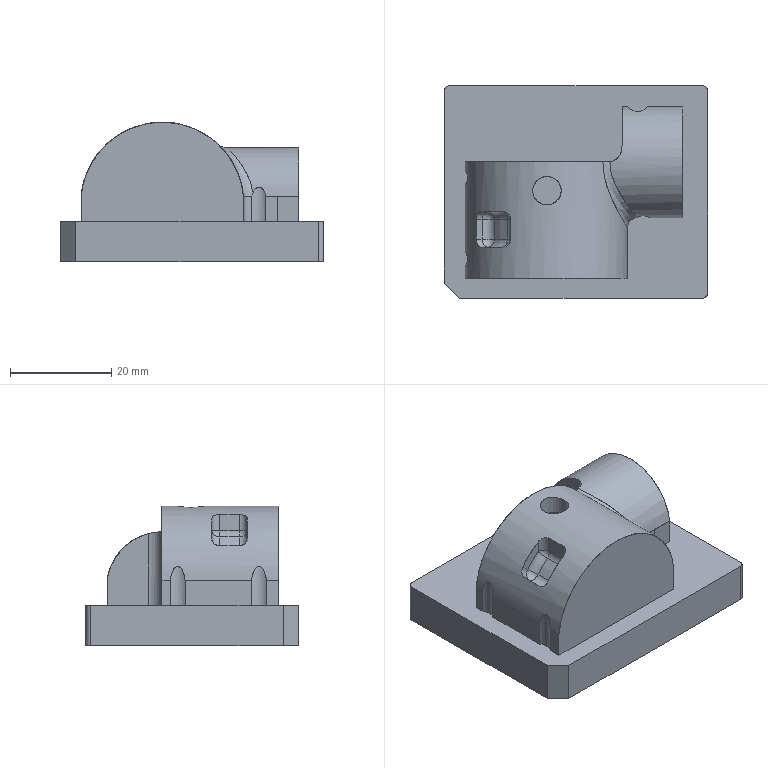CAM job | PowerMill | 3-axis milling, other | part box 52 x 42 x 27.622 mm
Tools:
number,name,type,diameter,tip_radius,length,cutting_length,overhang,flutes,holder,toolpaths_using
1,D10C,end_mill,10.0,0.0,60.0,,30.0,1,D42L35,2
2,D4C,end_mill,4.0,0.0,30.0,,15.0,1,D42L35,2
1,D10C_1_1_1,end_mill,10.0,0.0,60.0,,28.08,1,D42L35,3
2,D4C_1_1,end_mill,4.0,0.0,30.0,,19.8,1,D42L35,2
28,D2C_1_1,end_mill,2.0,0.0,4.16,,12.72,1,D42L35,1
3,D10_1_1_1,end_mill,10.0,0.0,60.0,,27.8,1,D42L35,6
7,R2_1_1,ball_nosed,4.0,2.0,30.0,,16.76,1,D42L35,1
10,D3_1_1,end_mill,3.0,0.0,30.0,,19.88,1,D42L35,1
4,R1_1_1,ball_nosed,2.0,1.0,5.0,,9.72,1,D42L35,2
13,Text_D4_1_1,taper_spherical,4.0,0.3,60.0,,19.88,1,D42L35,2
1,D10C_2_1_1,end_mill,10.0,0.0,60.0,,28.08,1,D42L35,3
2,D4C_2_1,end_mill,4.0,0.0,30.0,,19.68,1,D42L35,2
28,D2C_2_1,end_mill,2.0,0.0,4.24,,9.8,1,D42L35,1
7,R2_2_1,ball_nosed,4.0,2.0,30.0,,16.6,1,D42L35,1
10,D3_2_1,end_mill,3.0,0.0,30.0,,19.76,1,D42L35,1
Operations:
program,toolpath,strategy,tool,tool_number,tool_diameter,tip_radius,flutes,spindle_rpm,feed_cut,surface_speed_m_min_computed,feed_per_tooth_computed,tolerance,thickness,stepover,stepdown,cut_length,cut_time_min,total_time_min,workplane
04-S-2-F,精公开粗01-扫面平行-D10C,raster_area_clear,D10C_1_1_1,1,10.0,0.0,1.0,8000.0,10000.0,251.33,1.25,0.03,0.28,6.0,1.0,565.6,0.057,0.0629,
04-S-2-F,精公开粗01-外形偏置-D10C,offset_area_clear,D10C_1_1_1,1,10.0,0.0,1.0,8000.0,10000.0,251.33,1.25,0.03,0.28,6.0,1.0,24791.691,2.479,2.602,
04-S-2-F,精公开粗01-基准台等高-D10C,constantz,D10C_1_1_1,1,10.0,0.0,1.0,8000.0,10000.0,251.33,1.25,0.03,0.07,5.0,0.4,4769.097,0.477,0.49,
04-S-2-F,精公再粗02-外形偏置-D4C,offset_area_clear,D4C_1_1,2,4.0,0.0,1.0,18000.0,6000.0,226.19,0.3333,0.03,0.0,2.0,1.0,14887.954,2.481,2.559,
04-S-2-F,精公再粗02-平行中光-D4C,raster,D4C_1_1,2,4.0,0.0,1.0,18000.0,6000.0,226.19,0.3333,0.03,0.0,0.2,1.0,7797.636,1.3,1.36,
04-S-2-F,精公再粗03-外形偏置-D2C,offset_area_clear,D2C_1_1,28,2.0,0.0,1.0,18000.0,4000.0,113.1,0.2222,0.03,0.0,1.1,1.0,1024.756,0.256,0.5915,
04-S-2-F,精公基准台01-基准面偏置-D10,offset_area_clear,D10_1_1_1,3,10.0,0.0,1.0,8500.0,600.0,267.04,0.0706,0.005,0.38,5.0,1.0,295.104,0.492,0.514,
04-S-2-F,精公基准台01-外形侧光-D10,profile_area_clear,D10_1_1_1,3,10.0,0.0,1.0,8500.0,600.0,267.04,0.0706,0.005,-0.07,0.08,1.0,520.262,0.867,0.9659,
04-S-2-F,精公基准台01-基准台侧光-D10,profile_area_clear,D10_1_1_1,3,10.0,0.0,1.0,8500.0,600.0,267.04,0.0706,0.005,0.0,0.08,1.0,433.233,0.722,0.7895,
04-S-2-F,精公精光01-平行-R2,raster,R2_1_1,7,4.0,2.0,1.0,18000.0,2000.0,226.19,0.1111,0.005,-0.075,0.05,1.0,25834.296,12.917,13.018,
04-S-2-F,精公精光02-等高-D3,constantz,D3_1_1,10,3.0,0.0,1.0,18000.0,2000.0,169.65,0.1111,0.005,-0.075,5.0,0.03,9522.334,4.761,6.09,
04-S-2-F,精公精光03-三维偏置-R1,offset_3d,R1_1_1,4,2.0,1.0,1.0,18000.0,2000.0,113.1,0.1111,0.005,-0.075,0.03,1.0,2914.782,1.457,1.463,
04-S-2-F,精公刻字01-刻字-Text_D4,pattern,Text_D4_1_1,13,4.0,0.3,1.0,15000.0,1000.0,188.5,0.0667,0.005,0.0,5.0,1.0,56.018,0.056,0.0758,
04-S-2-R,粗公开粗01-扫面平行-D10C,raster_area_clear,D10C_2_1_1,1,10.0,0.0,1.0,8000.0,10000.0,251.33,1.25,0.03,0.15,6.0,1.0,563.0,0.056,0.0636,
04-S-2-R,粗公开粗01-外形偏置-D10C,offset_area_clear,D10C_2_1_1,1,10.0,0.0,1.0,8000.0,10000.0,251.33,1.25,0.03,0.15,6.0,1.0,24674.68,2.467,2.591,
04-S-2-R,粗公开粗01-基准台等高-D10C,constantz,D10C_2_1_1,1,10.0,0.0,1.0,8000.0,10000.0,251.33,1.25,0.03,0.07,5.0,0.4,4769.097,0.477,0.49,
04-S-2-R,粗公再粗02-外形偏置-D4C,offset_area_clear,D4C_2_1,2,4.0,0.0,1.0,18000.0,6000.0,226.19,0.3333,0.03,-0.13,2.0,1.0,14267.371,2.378,2.513,
04-S-2-R,粗公再粗02-平行中光-D4C,raster,D4C_2_1,2,4.0,0.0,1.0,18000.0,6000.0,226.19,0.3333,0.03,-0.13,0.2,1.0,7608.413,1.268,1.323,
04-S-2-R,粗公再粗03-外形偏置-D2C,offset_area_clear,D2C_2_1,28,2.0,0.0,1.0,18000.0,4000.0,113.1,0.2222,0.03,-0.13,1.1,1.0,972.061,0.243,0.5443,
04-S-2-R,粗公基准台01-基准面偏置-D10,offset_area_clear,D10_1_1_1,3,10.0,0.0,1.0,8500.0,600.0,267.04,0.0706,0.01,0.25,5.0,1.0,294.284,0.49,0.5126,
04-S-2-R,粗公基准台01-外形侧光-D10,profile_area_clear,D10_1_1_1,3,10.0,0.0,1.0,8500.0,600.0,267.04,0.0706,0.01,-0.2,0.08,1.0,518.278,0.864,0.9635,
04-S-2-R,粗公基准台01-基准台侧光-D10,profile_area_clear,D10_1_1_1,3,10.0,0.0,1.0,8500.0,600.0,267.04,0.0706,0.01,0.0,0.08,1.0,433.216,0.722,0.7895,
04-S-2-R,粗公精光01-平行-R2,raster,R2_2_1,7,4.0,2.0,1.0,18000.0,2000.0,226.19,0.1111,0.01,-0.205,0.06,1.0,21205.384,10.603,10.704,
04-S-2-R,粗公精光02-等高-D3,constantz,D3_2_1,10,3.0,0.0,1.0,18000.0,2000.0,169.65,0.1111,0.01,-0.205,5.0,0.036,8093.889,4.047,5.16,
04-S-2-R,粗公精光03-三维偏置-R1,offset_3d,R1_1_1,4,2.0,1.0,1.0,18000.0,2000.0,113.1,0.1111,0.01,-0.205,0.036,1.0,2575.828,1.288,1.294,
04-S-2-R,粗公刻字01-刻字-Text_D4,pattern,Text_D4_1_1,13,4.0,0.3,1.0,15000.0,1000.0,188.5,0.0667,0.01,0.0,5.0,1.0,56.414,0.056,0.0755,
,精公开粗01-外形偏置-D10C_Reference,offset_area_clear,D10C,1,10.0,0.0,1.0,8000.0,10000.0,251.33,1.25,0.03,0.28,6.0,1.0,49604.003,4.96,5.202,
,精公再粗02-外形偏置-D4C_Reference,offset_area_clear,D4C,2,4.0,0.0,1.0,18000.0,6000.0,226.19,0.3333,0.03,0.0,2.0,1.0,29071.976,4.845,4.927,
,粗公开粗01-外形偏置-D10C_Reference,offset_area_clear,D10C,1,10.0,0.0,1.0,8000.0,10000.0,251.33,1.25,0.03,0.15,6.0,1.0,49358.118,4.936,5.178,
,粗公再粗02-外形偏置-D4C_Reference,offset_area_clear,D4C,2,4.0,0.0,1.0,18000.0,6000.0,226.19,0.3333,0.03,-0.13,2.0,1.0,28158.12,4.693,4.793,